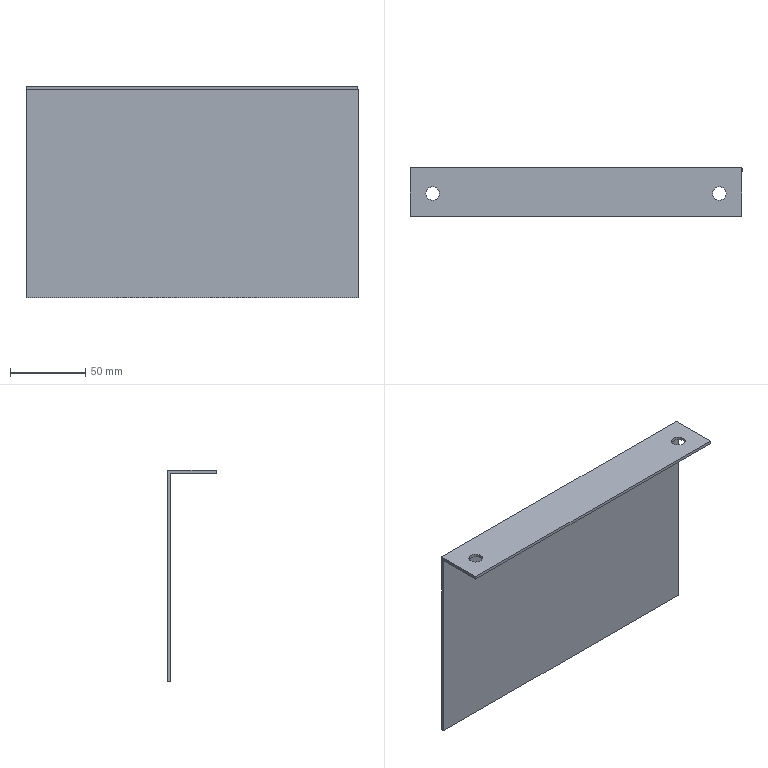Part | STEP file | lll_id2750_x_t | 1 solid | 10 faces | box 220 x 32 x 140 mm | volume 74546 mm3 | plane 8 | cylinder 2 | commonest cylinder face diameters 9 x2
STEP:
#1=CARTESIAN_POINT('',(3624.935,-391.,2.5));
#2=VERTEX_POINT('',#1);
#3=CARTESIAN_POINT('',(3624.935,-389.,2.5));
#4=VERTEX_POINT('',#3);
#5=CARTESIAN_POINT('',(3624.935,-391.,2.5));
#6=DIRECTION('',(0.,1.,0.));
#7=VECTOR('',#6,1.);
#8=LINE('',#5,#7);
#9=EDGE_CURVE('',#2,#4,#8,.T.);
#10=ORIENTED_EDGE('',*,*,#9,.T.);
#11=CARTESIAN_POINT('',(3844.935,-389.,2.5));
#12=VERTEX_POINT('',#11);
#13=CARTESIAN_POINT('',(3624.935,-389.,2.5));
#14=DIRECTION('',(1.,0.,0.));
#15=VECTOR('',#14,1.);
#16=LINE('',#13,#15);
#17=EDGE_CURVE('',#4,#12,#16,.T.);
#18=ORIENTED_EDGE('',*,*,#17,.T.);
#19=CARTESIAN_POINT('',(3844.935,-391.,2.5));
#20=VERTEX_POINT('',#19);
#21=CARTESIAN_POINT('',(3844.935,95.,2.5));
#22=DIRECTION('',(0.,1.,0.));
#23=VECTOR('',#22,1.);
#24=LINE('',#21,#23);
#25=EDGE_CURVE('',#20,#12,#24,.T.);
#26=ORIENTED_EDGE('',*,*,#25,.F.);
#27=CARTESIAN_POINT('',(3624.935,-391.,2.5));
#28=DIRECTION('',(1.,0.,0.));
#29=VECTOR('',#28,1.);
#30=LINE('',#27,#29);
#31=EDGE_CURVE('',#2,#20,#30,.T.);
#32=ORIENTED_EDGE('',*,*,#31,.F.);
#33=EDGE_LOOP('',(#10,#18,#26,#32));
#34=FACE_OUTER_BOUND('',#33,.T.);
#35=CARTESIAN_POINT('',(4817.435,95.,2.5));
#36=DIRECTION('',(0.,0.,-1.));
#37=DIRECTION('',(-1.,0.,0.));
#38=AXIS2_PLACEMENT_3D('',#35,#36,#37);
#39=PLANE('',#38);
#40=ADVANCED_FACE('',(#34),#39,.T.);
#41=CARTESIAN_POINT('',(3844.935,-391.,140.5));
#42=VERTEX_POINT('',#41);
#43=CARTESIAN_POINT('',(3624.935,-391.,140.5));
#44=VERTEX_POINT('',#43);
#45=CARTESIAN_POINT('',(3624.935,-391.,140.5));
#46=DIRECTION('',(-1.,0.,0.));
#47=VECTOR('',#46,1.);
#48=LINE('',#45,#47);
#49=EDGE_CURVE('',#42,#44,#48,.T.);
#50=ORIENTED_EDGE('',*,*,#49,.T.);
#51=CARTESIAN_POINT('',(3624.935,-391.,142.5));
#52=DIRECTION('',(0.,0.,-1.));
#53=VECTOR('',#52,1.);
#54=LINE('',#51,#53);
#55=EDGE_CURVE('',#44,#2,#54,.T.);
#56=ORIENTED_EDGE('',*,*,#55,.T.);
#57=ORIENTED_EDGE('',*,*,#31,.T.);
#58=CARTESIAN_POINT('',(3844.935,-391.,-78.5));
#59=DIRECTION('',(0.,0.,1.));
#60=VECTOR('',#59,1.);
#61=LINE('',#58,#60);
#62=EDGE_CURVE('',#20,#42,#61,.T.);
#63=ORIENTED_EDGE('',*,*,#62,.T.);
#64=EDGE_LOOP('',(#50,#56,#57,#63));
#65=FACE_OUTER_BOUND('',#64,.T.);
#66=CARTESIAN_POINT('',(3624.935,-391.,-78.5));
#67=DIRECTION('',(0.,1.,0.));
#68=DIRECTION('',(0.,0.,-1.));
#69=AXIS2_PLACEMENT_3D('',#66,#67,#68);
#70=PLANE('',#69);
#71=ADVANCED_FACE('',(#65),#70,.F.);
#72=CARTESIAN_POINT('',(3624.935,-389.,142.5));
#73=VERTEX_POINT('',#72);
#74=CARTESIAN_POINT('',(3624.935,-389.,-78.5));
#75=DIRECTION('',(0.,0.,-1.));
#76=VECTOR('',#75,1.);
#77=LINE('',#74,#76);
#78=EDGE_CURVE('',#73,#4,#77,.T.);
#79=ORIENTED_EDGE('',*,*,#78,.F.);
#80=CARTESIAN_POINT('',(3844.935,-389.,142.5));
#81=VERTEX_POINT('',#80);
#82=CARTESIAN_POINT('',(3624.935,-389.,142.5));
#83=DIRECTION('',(-1.,0.,0.));
#84=VECTOR('',#83,1.);
#85=LINE('',#82,#84);
#86=EDGE_CURVE('',#81,#73,#85,.T.);
#87=ORIENTED_EDGE('',*,*,#86,.F.);
#88=CARTESIAN_POINT('',(3844.935,-389.,-78.5));
#89=DIRECTION('',(0.,0.,1.));
#90=VECTOR('',#89,1.);
#91=LINE('',#88,#90);
#92=EDGE_CURVE('',#12,#81,#91,.T.);
#93=ORIENTED_EDGE('',*,*,#92,.F.);
#94=ORIENTED_EDGE('',*,*,#17,.F.);
#95=EDGE_LOOP('',(#79,#87,#93,#94));
#96=FACE_OUTER_BOUND('',#95,.T.);
#97=CARTESIAN_POINT('',(3624.935,-389.,-78.5));
#98=DIRECTION('',(0.,1.,0.));
#99=DIRECTION('',(0.,0.,-1.));
#100=AXIS2_PLACEMENT_3D('',#97,#98,#99);
#101=PLANE('',#100);
#102=ADVANCED_FACE('',(#96),#101,.T.);
#103=ORIENTED_EDGE('',*,*,#9,.F.);
#104=ORIENTED_EDGE('',*,*,#55,.F.);
#105=CARTESIAN_POINT('',(3624.935,-421.,140.5));
#106=VERTEX_POINT('',#105);
#107=CARTESIAN_POINT('',(3624.935,-391.,140.5));
#108=DIRECTION('',(0.,1.,0.));
#109=VECTOR('',#108,1.);
#110=LINE('',#107,#109);
#111=EDGE_CURVE('',#106,#44,#110,.T.);
#112=ORIENTED_EDGE('',*,*,#111,.F.);
#113=CARTESIAN_POINT('',(3624.935,-421.,142.5));
#114=VERTEX_POINT('',#113);
#115=CARTESIAN_POINT('',(3624.935,-421.,142.5));
#116=DIRECTION('',(0.,0.,-1.));
#117=VECTOR('',#116,1.);
#118=LINE('',#115,#117);
#119=EDGE_CURVE('',#114,#106,#118,.T.);
#120=ORIENTED_EDGE('',*,*,#119,.F.);
#121=CARTESIAN_POINT('',(3624.935,-391.,142.5));
#122=DIRECTION('',(0.,1.,0.));
#123=VECTOR('',#122,1.);
#124=LINE('',#121,#123);
#125=EDGE_CURVE('',#114,#73,#124,.T.);
#126=ORIENTED_EDGE('',*,*,#125,.T.);
#127=ORIENTED_EDGE('',*,*,#78,.T.);
#128=EDGE_LOOP('',(#103,#104,#112,#120,#126,#127));
#129=FACE_OUTER_BOUND('',#128,.T.);
#130=CARTESIAN_POINT('',(3624.935,-391.,142.5));
#131=DIRECTION('',(-1.,0.,0.));
#132=DIRECTION('',(0.,0.,-1.));
#133=AXIS2_PLACEMENT_3D('',#130,#131,#132);
#134=PLANE('',#133);
#135=ADVANCED_FACE('',(#129),#134,.T.);
#136=ORIENTED_EDGE('',*,*,#119,.T.);
#137=CARTESIAN_POINT('',(3844.935,-421.,140.5));
#138=VERTEX_POINT('',#137);
#139=CARTESIAN_POINT('',(3624.935,-421.,140.5));
#140=DIRECTION('',(-1.,0.,0.));
#141=VECTOR('',#140,1.);
#142=LINE('',#139,#141);
#143=EDGE_CURVE('',#138,#106,#142,.T.);
#144=ORIENTED_EDGE('',*,*,#143,.F.);
#145=CARTESIAN_POINT('',(3844.935,-421.,142.5));
#146=VERTEX_POINT('',#145);
#147=CARTESIAN_POINT('',(3844.935,-421.,142.5));
#148=DIRECTION('',(0.,0.,-1.));
#149=VECTOR('',#148,1.);
#150=LINE('',#147,#149);
#151=EDGE_CURVE('',#146,#138,#150,.T.);
#152=ORIENTED_EDGE('',*,*,#151,.F.);
#153=CARTESIAN_POINT('',(3624.935,-421.,142.5));
#154=DIRECTION('',(-1.,0.,0.));
#155=VECTOR('',#154,1.);
#156=LINE('',#153,#155);
#157=EDGE_CURVE('',#146,#114,#156,.T.);
#158=ORIENTED_EDGE('',*,*,#157,.T.);
#159=EDGE_LOOP('',(#136,#144,#152,#158));
#160=FACE_OUTER_BOUND('',#159,.T.);
#161=CARTESIAN_POINT('',(3624.935,-421.,142.5));
#162=DIRECTION('',(0.,-1.,0.));
#163=DIRECTION('',(1.,0.,0.));
#164=AXIS2_PLACEMENT_3D('',#161,#162,#163);
#165=PLANE('',#164);
#166=ADVANCED_FACE('',(#160),#165,.T.);
#167=CARTESIAN_POINT('',(3844.935,-391.,142.5));
#168=DIRECTION('',(0.,1.,0.));
#169=VECTOR('',#168,1.);
#170=LINE('',#167,#169);
#171=EDGE_CURVE('',#146,#81,#170,.T.);
#172=ORIENTED_EDGE('',*,*,#171,.F.);
#173=ORIENTED_EDGE('',*,*,#151,.T.);
#174=CARTESIAN_POINT('',(3844.935,-391.,140.5));
#175=DIRECTION('',(0.,1.,0.));
#176=VECTOR('',#175,1.);
#177=LINE('',#174,#176);
#178=EDGE_CURVE('',#138,#42,#177,.T.);
#179=ORIENTED_EDGE('',*,*,#178,.T.);
#180=ORIENTED_EDGE('',*,*,#62,.F.);
#181=ORIENTED_EDGE('',*,*,#25,.T.);
#182=ORIENTED_EDGE('',*,*,#92,.T.);
#183=EDGE_LOOP('',(#172,#173,#179,#180,#181,#182));
#184=FACE_OUTER_BOUND('',#183,.T.);
#185=CARTESIAN_POINT('',(3844.935,-391.,-78.5));
#186=DIRECTION('',(-1.,0.,0.));
#187=DIRECTION('',(0.,0.,-1.));
#188=AXIS2_PLACEMENT_3D('',#185,#186,#187);
#189=PLANE('',#188);
#190=ADVANCED_FACE('',(#184),#189,.F.);
#191=CARTESIAN_POINT('',(3825.435,-406.,142.5));
#192=VERTEX_POINT('',#191);
#193=CARTESIAN_POINT('',(3829.935,-406.,142.5));
#194=DIRECTION('',(0.,0.,-1.));
#195=DIRECTION('',(-1.,0.,0.));
#196=AXIS2_PLACEMENT_3D('',#193,#194,#195);
#197=CIRCLE('',#196,4.5);
#198=EDGE_CURVE('',#192,#192,#197,.T.);
#199=ORIENTED_EDGE('',*,*,#198,.F.);
#200=EDGE_LOOP('',(#199));
#201=FACE_BOUND('',#200,.T.);
#202=CARTESIAN_POINT('',(3834.435,-406.,140.5));
#203=VERTEX_POINT('',#202);
#204=CARTESIAN_POINT('',(3829.935,-406.,140.5));
#205=DIRECTION('',(0.,0.,-1.));
#206=DIRECTION('',(1.,0.,0.));
#207=AXIS2_PLACEMENT_3D('',#204,#205,#206);
#208=CIRCLE('',#207,4.5);
#209=EDGE_CURVE('',#203,#203,#208,.T.);
#210=ORIENTED_EDGE('',*,*,#209,.T.);
#211=EDGE_LOOP('',(#210));
#212=FACE_BOUND('',#211,.T.);
#213=CARTESIAN_POINT('',(3829.935,-406.,140.5));
#214=DIRECTION('',(0.,0.,1.));
#215=DIRECTION('',(1.,0.,0.));
#216=AXIS2_PLACEMENT_3D('',#213,#214,#215);
#217=CYLINDRICAL_SURFACE('',#216,4.5);
#218=ADVANCED_FACE('',(#201,#212),#217,.F.);
#219=CARTESIAN_POINT('',(3635.435,-406.,142.5));
#220=VERTEX_POINT('',#219);
#221=CARTESIAN_POINT('',(3639.935,-406.,142.5));
#222=DIRECTION('',(0.,0.,-1.));
#223=DIRECTION('',(-1.,0.,0.));
#224=AXIS2_PLACEMENT_3D('',#221,#222,#223);
#225=CIRCLE('',#224,4.5);
#226=EDGE_CURVE('',#220,#220,#225,.T.);
#227=ORIENTED_EDGE('',*,*,#226,.F.);
#228=EDGE_LOOP('',(#227));
#229=FACE_BOUND('',#228,.T.);
#230=CARTESIAN_POINT('',(3635.435,-406.,140.5));
#231=VERTEX_POINT('',#230);
#232=CARTESIAN_POINT('',(3639.935,-406.,140.5));
#233=DIRECTION('',(0.,0.,-1.));
#234=DIRECTION('',(-1.,0.,0.));
#235=AXIS2_PLACEMENT_3D('',#232,#233,#234);
#236=CIRCLE('',#235,4.5);
#237=EDGE_CURVE('',#231,#231,#236,.T.);
#238=ORIENTED_EDGE('',*,*,#237,.T.);
#239=EDGE_LOOP('',(#238));
#240=FACE_BOUND('',#239,.T.);
#241=CARTESIAN_POINT('',(3639.935,-406.,140.5));
#242=DIRECTION('',(0.,0.,1.));
#243=DIRECTION('',(-1.,0.,0.));
#244=AXIS2_PLACEMENT_3D('',#241,#242,#243);
#245=CYLINDRICAL_SURFACE('',#244,4.5);
#246=ADVANCED_FACE('',(#229,#240),#245,.F.);
#247=ORIENTED_EDGE('',*,*,#226,.T.);
#248=EDGE_LOOP('',(#247));
#249=FACE_BOUND('',#248,.T.);
#250=ORIENTED_EDGE('',*,*,#198,.T.);
#251=EDGE_LOOP('',(#250));
#252=FACE_BOUND('',#251,.T.);
#253=ORIENTED_EDGE('',*,*,#171,.T.);
#254=ORIENTED_EDGE('',*,*,#86,.T.);
#255=ORIENTED_EDGE('',*,*,#125,.F.);
#256=ORIENTED_EDGE('',*,*,#157,.F.);
#257=EDGE_LOOP('',(#253,#254,#255,#256));
#258=FACE_BOUND('',#257,.T.);
#259=CARTESIAN_POINT('',(3624.935,-391.,142.5));
#260=DIRECTION('',(0.,0.,-1.));
#261=DIRECTION('',(1.,0.,0.));
#262=AXIS2_PLACEMENT_3D('',#259,#260,#261);
#263=PLANE('',#262);
#264=ADVANCED_FACE('',(#249,#252,#258),#263,.F.);
#265=ORIENTED_EDGE('',*,*,#237,.F.);
#266=EDGE_LOOP('',(#265));
#267=FACE_BOUND('',#266,.T.);
#268=ORIENTED_EDGE('',*,*,#209,.F.);
#269=EDGE_LOOP('',(#268));
#270=FACE_BOUND('',#269,.T.);
#271=ORIENTED_EDGE('',*,*,#178,.F.);
#272=ORIENTED_EDGE('',*,*,#143,.T.);
#273=ORIENTED_EDGE('',*,*,#111,.T.);
#274=ORIENTED_EDGE('',*,*,#49,.F.);
#275=EDGE_LOOP('',(#271,#272,#273,#274));
#276=FACE_BOUND('',#275,.T.);
#277=CARTESIAN_POINT('',(3624.935,-391.,140.5));
#278=DIRECTION('',(0.,0.,-1.));
#279=DIRECTION('',(1.,0.,0.));
#280=AXIS2_PLACEMENT_3D('',#277,#278,#279);
#281=PLANE('',#280);
#282=ADVANCED_FACE('',(#267,#270,#276),#281,.T.);
#283=CLOSED_SHELL('',(#40,#71,#102,#135,#166,#190,#218,#246,#264,#282));
#284=MANIFOLD_SOLID_BREP('',#283);
#285=(LENGTH_UNIT()NAMED_UNIT(*)SI_UNIT(.MILLI.,.METRE.));
#286=UNCERTAINTY_MEASURE_WITH_UNIT(LENGTH_MEASURE(0.00002),#285,'','');
#287=(NAMED_UNIT(*)PLANE_ANGLE_UNIT()SI_UNIT($,.RADIAN.));
#288=PLANE_ANGLE_MEASURE_WITH_UNIT(PLANE_ANGLE_MEASURE(0.01745),#287);
#289=DIMENSIONAL_EXPONENTS(0.,0.,0.,0.,0.,0.,0.);
#290=(CONVERSION_BASED_UNIT('DEGREE',#288)NAMED_UNIT(#289)PLANE_ANGLE_UNIT());
#291=(NAMED_UNIT(*)SI_UNIT($,.STERADIAN.)SOLID_ANGLE_UNIT());
#292=(GEOMETRIC_REPRESENTATION_CONTEXT(3)GLOBAL_UNCERTAINTY_ASSIGNED_CONTEXT((#286))GLOBAL_UNIT_ASSIGNED_CONTEXT((#285,#290,#291))REPRESENTATION_CONTEXT('',''));
#293=ADVANCED_BREP_SHAPE_REPRESENTATION('',(#284),#292);